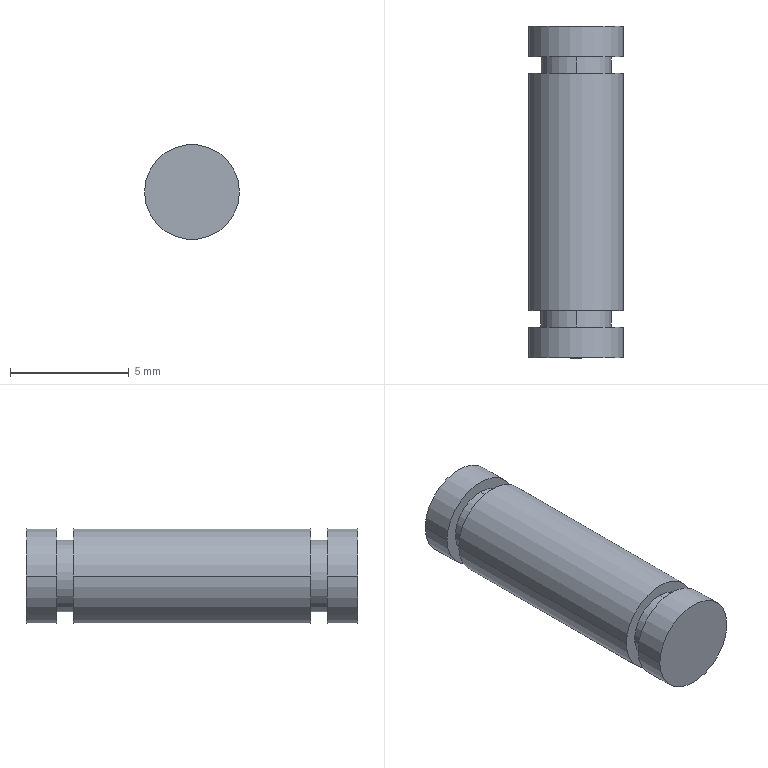Part | NX | 1 solid | 16 faces | box 4 x 14 x 4 mm | volume 168.232 mm3 | cylinder 10 | plane 6 | commonest cylinder face diameters 4 x6 3 x4
STEP:
#1=CARTESIAN_POINT('',(-42.,151.,-84.4));
#2=VERTEX_POINT('',#1);
#3=CARTESIAN_POINT('',(-46.,151.,-84.4));
#4=VERTEX_POINT('',#3);
#5=CARTESIAN_POINT('',(-44.,151.,-84.4));
#6=DIRECTION('',(0.,1.,0.));
#7=DIRECTION('',(-1.,0.,0.));
#8=AXIS2_PLACEMENT_3D('',#5,#6,#7);
#9=CIRCLE('',#8,2.);
#10=EDGE_CURVE('',#2,#4,#9,.T.);
#11=ORIENTED_EDGE('',*,*,#10,.T.);
#12=CARTESIAN_POINT('',(-46.,152.3,-84.4));
#13=VERTEX_POINT('',#12);
#14=CARTESIAN_POINT('',(-46.,165.,-84.4));
#15=DIRECTION('',(0.,1.,0.));
#16=VECTOR('',#15,1000.);
#17=LINE('',#14,#16);
#18=EDGE_CURVE('',#4,#13,#17,.T.);
#19=ORIENTED_EDGE('',*,*,#18,.T.);
#20=CARTESIAN_POINT('',(-42.,152.3,-84.4));
#21=VERTEX_POINT('',#20);
#22=CARTESIAN_POINT('',(-44.,152.3,-84.4));
#23=DIRECTION('',(0.,1.,0.));
#24=DIRECTION('',(-1.,0.,0.));
#25=AXIS2_PLACEMENT_3D('',#22,#23,#24);
#26=CIRCLE('',#25,2.);
#27=EDGE_CURVE('',#21,#13,#26,.T.);
#28=ORIENTED_EDGE('',*,*,#27,.F.);
#29=CARTESIAN_POINT('',(-42.,165.,-84.4));
#30=DIRECTION('',(0.,1.,0.));
#31=VECTOR('',#30,1000.);
#32=LINE('',#29,#31);
#33=EDGE_CURVE('',#2,#21,#32,.T.);
#34=ORIENTED_EDGE('',*,*,#33,.F.);
#35=EDGE_LOOP('',(#11,#19,#28,#34));
#36=FACE_BOUND('',#35,.T.);
#37=CARTESIAN_POINT('',(-44.,165.,-84.4));
#38=DIRECTION('',(0.,1.,0.));
#39=DIRECTION('',(-1.,0.,0.));
#40=AXIS2_PLACEMENT_3D('',#37,#38,#39);
#41=CYLINDRICAL_SURFACE('',#40,2.);
#42=ADVANCED_FACE('',(#36),#41,.T.);
#43=CARTESIAN_POINT('',(-42.,163.7,-84.4));
#44=VERTEX_POINT('',#43);
#45=CARTESIAN_POINT('',(-46.,163.7,-84.4));
#46=VERTEX_POINT('',#45);
#47=CARTESIAN_POINT('',(-44.,163.7,-84.4));
#48=DIRECTION('',(0.,1.,0.));
#49=DIRECTION('',(-1.,0.,0.));
#50=AXIS2_PLACEMENT_3D('',#47,#48,#49);
#51=CIRCLE('',#50,2.);
#52=EDGE_CURVE('',#44,#46,#51,.T.);
#53=ORIENTED_EDGE('',*,*,#52,.T.);
#54=CARTESIAN_POINT('',(-46.,165.,-84.4));
#55=VERTEX_POINT('',#54);
#56=CARTESIAN_POINT('',(-46.,165.,-84.4));
#57=DIRECTION('',(0.,1.,0.));
#58=VECTOR('',#57,1000.);
#59=LINE('',#56,#58);
#60=EDGE_CURVE('',#55,#46,#59,.F.);
#61=ORIENTED_EDGE('',*,*,#60,.F.);
#62=CARTESIAN_POINT('',(-42.,165.,-84.4));
#63=VERTEX_POINT('',#62);
#64=CARTESIAN_POINT('',(-44.,165.,-84.4));
#65=DIRECTION('',(0.,1.,0.));
#66=DIRECTION('',(-1.,0.,0.));
#67=AXIS2_PLACEMENT_3D('',#64,#65,#66);
#68=CIRCLE('',#67,2.);
#69=EDGE_CURVE('',#63,#55,#68,.T.);
#70=ORIENTED_EDGE('',*,*,#69,.F.);
#71=CARTESIAN_POINT('',(-42.,165.,-84.4));
#72=DIRECTION('',(0.,1.,0.));
#73=VECTOR('',#72,1000.);
#74=LINE('',#71,#73);
#75=EDGE_CURVE('',#63,#44,#74,.F.);
#76=ORIENTED_EDGE('',*,*,#75,.T.);
#77=EDGE_LOOP('',(#53,#61,#70,#76));
#78=FACE_BOUND('',#77,.T.);
#79=CARTESIAN_POINT('',(-44.,165.,-84.4));
#80=DIRECTION('',(0.,1.,0.));
#81=DIRECTION('',(-1.,0.,0.));
#82=AXIS2_PLACEMENT_3D('',#79,#80,#81);
#83=CYLINDRICAL_SURFACE('',#82,2.);
#84=ADVANCED_FACE('',(#78),#83,.T.);
#85=CARTESIAN_POINT('',(-42.,153.,-84.4));
#86=VERTEX_POINT('',#85);
#87=CARTESIAN_POINT('',(-46.,153.,-84.4));
#88=VERTEX_POINT('',#87);
#89=CARTESIAN_POINT('',(-44.,153.,-84.4));
#90=DIRECTION('',(0.,1.,0.));
#91=DIRECTION('',(-1.,0.,0.));
#92=AXIS2_PLACEMENT_3D('',#89,#90,#91);
#93=CIRCLE('',#92,2.);
#94=EDGE_CURVE('',#86,#88,#93,.T.);
#95=ORIENTED_EDGE('',*,*,#94,.T.);
#96=CARTESIAN_POINT('',(-46.,163.,-84.4));
#97=VERTEX_POINT('',#96);
#98=CARTESIAN_POINT('',(-46.,165.,-84.4));
#99=DIRECTION('',(0.,1.,0.));
#100=VECTOR('',#99,1000.);
#101=LINE('',#98,#100);
#102=EDGE_CURVE('',#97,#88,#101,.F.);
#103=ORIENTED_EDGE('',*,*,#102,.F.);
#104=CARTESIAN_POINT('',(-42.,163.,-84.4));
#105=VERTEX_POINT('',#104);
#106=CARTESIAN_POINT('',(-44.,163.,-84.4));
#107=DIRECTION('',(0.,1.,0.));
#108=DIRECTION('',(-1.,0.,0.));
#109=AXIS2_PLACEMENT_3D('',#106,#107,#108);
#110=CIRCLE('',#109,2.);
#111=EDGE_CURVE('',#105,#97,#110,.T.);
#112=ORIENTED_EDGE('',*,*,#111,.F.);
#113=CARTESIAN_POINT('',(-42.,165.,-84.4));
#114=DIRECTION('',(0.,1.,0.));
#115=VECTOR('',#114,1000.);
#116=LINE('',#113,#115);
#117=EDGE_CURVE('',#105,#86,#116,.F.);
#118=ORIENTED_EDGE('',*,*,#117,.T.);
#119=EDGE_LOOP('',(#95,#103,#112,#118));
#120=FACE_BOUND('',#119,.T.);
#121=CARTESIAN_POINT('',(-44.,165.,-84.4));
#122=DIRECTION('',(0.,1.,0.));
#123=DIRECTION('',(-1.,0.,0.));
#124=AXIS2_PLACEMENT_3D('',#121,#122,#123);
#125=CYLINDRICAL_SURFACE('',#124,2.);
#126=ADVANCED_FACE('',(#120),#125,.T.);
#127=ORIENTED_EDGE('',*,*,#52,.F.);
#128=CARTESIAN_POINT('',(-44.,163.7,-84.4));
#129=DIRECTION('',(0.,1.,0.));
#130=DIRECTION('',(-1.,0.,0.));
#131=AXIS2_PLACEMENT_3D('',#128,#129,#130);
#132=CIRCLE('',#131,2.);
#133=EDGE_CURVE('',#46,#44,#132,.T.);
#134=ORIENTED_EDGE('',*,*,#133,.F.);
#135=EDGE_LOOP('',(#127,#134));
#136=FACE_BOUND('',#135,.T.);
#137=CARTESIAN_POINT('',(-44.,163.7,-82.9));
#138=VERTEX_POINT('',#137);
#139=CARTESIAN_POINT('',(-44.,163.7,-85.9));
#140=VERTEX_POINT('',#139);
#141=CARTESIAN_POINT('',(-44.,163.7,-84.4));
#142=DIRECTION('',(0.,1.,0.));
#143=DIRECTION('',(1.,0.,0.));
#144=AXIS2_PLACEMENT_3D('',#141,#142,#143);
#145=CIRCLE('',#144,1.5);
#146=EDGE_CURVE('',#138,#140,#145,.T.);
#147=ORIENTED_EDGE('',*,*,#146,.T.);
#148=CARTESIAN_POINT('',(-44.,163.7,-84.4));
#149=DIRECTION('',(0.,1.,0.));
#150=DIRECTION('',(1.,0.,0.));
#151=AXIS2_PLACEMENT_3D('',#148,#149,#150);
#152=CIRCLE('',#151,1.5);
#153=EDGE_CURVE('',#140,#138,#152,.T.);
#154=ORIENTED_EDGE('',*,*,#153,.T.);
#155=EDGE_LOOP('',(#147,#154));
#156=FACE_BOUND('',#155,.T.);
#157=CARTESIAN_POINT('',(-41.314,163.7,-84.4));
#158=DIRECTION('',(0.,1.,0.));
#159=DIRECTION('',(0.,0.,-1.));
#160=AXIS2_PLACEMENT_3D('',#157,#158,#159);
#161=PLANE('',#160);
#162=ADVANCED_FACE('',(#136,#156),#161,.F.);
#163=ORIENTED_EDGE('',*,*,#146,.F.);
#164=CARTESIAN_POINT('',(-44.,163.,-82.9));
#165=VERTEX_POINT('',#164);
#166=CARTESIAN_POINT('',(-44.,163.35,-82.9));
#167=DIRECTION('',(0.,1.,0.));
#168=VECTOR('',#167,1000.);
#169=LINE('',#166,#168);
#170=EDGE_CURVE('',#165,#138,#169,.T.);
#171=ORIENTED_EDGE('',*,*,#170,.F.);
#172=CARTESIAN_POINT('',(-44.,163.,-85.9));
#173=VERTEX_POINT('',#172);
#174=CARTESIAN_POINT('',(-44.,163.,-84.4));
#175=DIRECTION('',(0.,1.,0.));
#176=DIRECTION('',(1.,0.,0.));
#177=AXIS2_PLACEMENT_3D('',#174,#175,#176);
#178=CIRCLE('',#177,1.5);
#179=EDGE_CURVE('',#165,#173,#178,.T.);
#180=ORIENTED_EDGE('',*,*,#179,.T.);
#181=CARTESIAN_POINT('',(-44.,163.35,-85.9));
#182=DIRECTION('',(0.,1.,0.));
#183=VECTOR('',#182,1000.);
#184=LINE('',#181,#183);
#185=EDGE_CURVE('',#173,#140,#184,.T.);
#186=ORIENTED_EDGE('',*,*,#185,.T.);
#187=EDGE_LOOP('',(#163,#171,#180,#186));
#188=FACE_BOUND('',#187,.T.);
#189=CARTESIAN_POINT('',(-44.,163.35,-84.4));
#190=DIRECTION('',(0.,1.,0.));
#191=DIRECTION('',(0.,0.,1.));
#192=AXIS2_PLACEMENT_3D('',#189,#190,#191);
#193=CYLINDRICAL_SURFACE('',#192,1.5);
#194=ADVANCED_FACE('',(#188),#193,.T.);
#195=CARTESIAN_POINT('',(-44.,163.,-84.4));
#196=DIRECTION('',(0.,1.,0.));
#197=DIRECTION('',(-1.,0.,0.));
#198=AXIS2_PLACEMENT_3D('',#195,#196,#197);
#199=CIRCLE('',#198,2.);
#200=EDGE_CURVE('',#97,#105,#199,.T.);
#201=ORIENTED_EDGE('',*,*,#200,.T.);
#202=ORIENTED_EDGE('',*,*,#111,.T.);
#203=EDGE_LOOP('',(#201,#202));
#204=FACE_BOUND('',#203,.T.);
#205=ORIENTED_EDGE('',*,*,#179,.F.);
#206=CARTESIAN_POINT('',(-44.,163.,-84.4));
#207=DIRECTION('',(0.,1.,0.));
#208=DIRECTION('',(1.,0.,0.));
#209=AXIS2_PLACEMENT_3D('',#206,#207,#208);
#210=CIRCLE('',#209,1.5);
#211=EDGE_CURVE('',#173,#165,#210,.T.);
#212=ORIENTED_EDGE('',*,*,#211,.F.);
#213=EDGE_LOOP('',(#205,#212));
#214=FACE_BOUND('',#213,.T.);
#215=CARTESIAN_POINT('',(-42.25,163.,-84.4));
#216=DIRECTION('',(0.,-1.,0.));
#217=DIRECTION('',(-1.,0.,0.));
#218=AXIS2_PLACEMENT_3D('',#215,#216,#217);
#219=PLANE('',#218);
#220=ADVANCED_FACE('',(#204,#214),#219,.F.);
#221=ORIENTED_EDGE('',*,*,#94,.F.);
#222=CARTESIAN_POINT('',(-44.,153.,-84.4));
#223=DIRECTION('',(0.,1.,0.));
#224=DIRECTION('',(-1.,0.,0.));
#225=AXIS2_PLACEMENT_3D('',#222,#223,#224);
#226=CIRCLE('',#225,2.);
#227=EDGE_CURVE('',#88,#86,#226,.T.);
#228=ORIENTED_EDGE('',*,*,#227,.F.);
#229=EDGE_LOOP('',(#221,#228));
#230=FACE_BOUND('',#229,.T.);
#231=CARTESIAN_POINT('',(-44.,153.,-85.9));
#232=VERTEX_POINT('',#231);
#233=CARTESIAN_POINT('',(-44.,153.,-82.9));
#234=VERTEX_POINT('',#233);
#235=CARTESIAN_POINT('',(-44.,153.,-84.4));
#236=DIRECTION('',(0.,1.,0.));
#237=DIRECTION('',(0.,0.,1.));
#238=AXIS2_PLACEMENT_3D('',#235,#236,#237);
#239=CIRCLE('',#238,1.5);
#240=EDGE_CURVE('',#232,#234,#239,.T.);
#241=ORIENTED_EDGE('',*,*,#240,.T.);
#242=CARTESIAN_POINT('',(-44.,153.,-84.4));
#243=DIRECTION('',(0.,1.,0.));
#244=DIRECTION('',(0.,0.,1.));
#245=AXIS2_PLACEMENT_3D('',#242,#243,#244);
#246=CIRCLE('',#245,1.5);
#247=EDGE_CURVE('',#234,#232,#246,.T.);
#248=ORIENTED_EDGE('',*,*,#247,.T.);
#249=EDGE_LOOP('',(#241,#248));
#250=FACE_BOUND('',#249,.T.);
#251=CARTESIAN_POINT('',(-42.25,153.,-84.4));
#252=DIRECTION('',(0.,1.,0.));
#253=DIRECTION('',(0.,0.,-1.));
#254=AXIS2_PLACEMENT_3D('',#251,#252,#253);
#255=PLANE('',#254);
#256=ADVANCED_FACE('',(#230,#250),#255,.F.);
#257=ORIENTED_EDGE('',*,*,#240,.F.);
#258=CARTESIAN_POINT('',(-44.,152.3,-85.9));
#259=VERTEX_POINT('',#258);
#260=CARTESIAN_POINT('',(-44.,154.65,-85.9));
#261=DIRECTION('',(0.,1.,0.));
#262=VECTOR('',#261,1000.);
#263=LINE('',#260,#262);
#264=EDGE_CURVE('',#259,#232,#263,.T.);
#265=ORIENTED_EDGE('',*,*,#264,.F.);
#266=CARTESIAN_POINT('',(-44.,152.3,-82.9));
#267=VERTEX_POINT('',#266);
#268=CARTESIAN_POINT('',(-44.,152.3,-84.4));
#269=DIRECTION('',(0.,1.,0.));
#270=DIRECTION('',(0.,0.,1.));
#271=AXIS2_PLACEMENT_3D('',#268,#269,#270);
#272=CIRCLE('',#271,1.5);
#273=EDGE_CURVE('',#259,#267,#272,.T.);
#274=ORIENTED_EDGE('',*,*,#273,.T.);
#275=CARTESIAN_POINT('',(-44.,154.65,-82.9));
#276=DIRECTION('',(0.,1.,0.));
#277=VECTOR('',#276,1000.);
#278=LINE('',#275,#277);
#279=EDGE_CURVE('',#267,#234,#278,.T.);
#280=ORIENTED_EDGE('',*,*,#279,.T.);
#281=EDGE_LOOP('',(#257,#265,#274,#280));
#282=FACE_BOUND('',#281,.T.);
#283=CARTESIAN_POINT('',(-44.,154.65,-84.4));
#284=DIRECTION('',(0.,1.,0.));
#285=DIRECTION('',(0.,0.,1.));
#286=AXIS2_PLACEMENT_3D('',#283,#284,#285);
#287=CYLINDRICAL_SURFACE('',#286,1.5);
#288=ADVANCED_FACE('',(#282),#287,.T.);
#289=ORIENTED_EDGE('',*,*,#27,.T.);
#290=CARTESIAN_POINT('',(-44.,152.3,-84.4));
#291=DIRECTION('',(0.,1.,0.));
#292=DIRECTION('',(-1.,0.,0.));
#293=AXIS2_PLACEMENT_3D('',#290,#291,#292);
#294=CIRCLE('',#293,2.);
#295=EDGE_CURVE('',#13,#21,#294,.T.);
#296=ORIENTED_EDGE('',*,*,#295,.T.);
#297=EDGE_LOOP('',(#289,#296));
#298=FACE_BOUND('',#297,.T.);
#299=ORIENTED_EDGE('',*,*,#273,.F.);
#300=CARTESIAN_POINT('',(-44.,152.3,-84.4));
#301=DIRECTION('',(0.,1.,0.));
#302=DIRECTION('',(0.,0.,1.));
#303=AXIS2_PLACEMENT_3D('',#300,#301,#302);
#304=CIRCLE('',#303,1.5);
#305=EDGE_CURVE('',#267,#259,#304,.T.);
#306=ORIENTED_EDGE('',*,*,#305,.F.);
#307=EDGE_LOOP('',(#299,#306));
#308=FACE_BOUND('',#307,.T.);
#309=CARTESIAN_POINT('',(-41.396,152.3,-84.4));
#310=DIRECTION('',(0.,1.,0.));
#311=DIRECTION('',(0.,0.,-1.));
#312=AXIS2_PLACEMENT_3D('',#309,#310,#311);
#313=PLANE('',#312);
#314=ADVANCED_FACE('',(#298,#308),#313,.T.);
#315=ORIENTED_EDGE('',*,*,#200,.F.);
#316=ORIENTED_EDGE('',*,*,#102,.T.);
#317=ORIENTED_EDGE('',*,*,#227,.T.);
#318=ORIENTED_EDGE('',*,*,#117,.F.);
#319=EDGE_LOOP('',(#315,#316,#317,#318));
#320=FACE_BOUND('',#319,.T.);
#321=CARTESIAN_POINT('',(-44.,165.,-84.4));
#322=DIRECTION('',(0.,1.,0.));
#323=DIRECTION('',(-1.,0.,0.));
#324=AXIS2_PLACEMENT_3D('',#321,#322,#323);
#325=CYLINDRICAL_SURFACE('',#324,2.);
#326=ADVANCED_FACE('',(#320),#325,.T.);
#327=ORIENTED_EDGE('',*,*,#279,.F.);
#328=ORIENTED_EDGE('',*,*,#305,.T.);
#329=ORIENTED_EDGE('',*,*,#264,.T.);
#330=ORIENTED_EDGE('',*,*,#247,.F.);
#331=EDGE_LOOP('',(#327,#328,#329,#330));
#332=FACE_BOUND('',#331,.T.);
#333=CARTESIAN_POINT('',(-44.,154.65,-84.4));
#334=DIRECTION('',(0.,1.,0.));
#335=DIRECTION('',(0.,0.,1.));
#336=AXIS2_PLACEMENT_3D('',#333,#334,#335);
#337=CYLINDRICAL_SURFACE('',#336,1.5);
#338=ADVANCED_FACE('',(#332),#337,.T.);
#339=ORIENTED_EDGE('',*,*,#60,.T.);
#340=ORIENTED_EDGE('',*,*,#133,.T.);
#341=ORIENTED_EDGE('',*,*,#75,.F.);
#342=CARTESIAN_POINT('',(-44.,165.,-84.4));
#343=DIRECTION('',(0.,1.,0.));
#344=DIRECTION('',(-1.,0.,0.));
#345=AXIS2_PLACEMENT_3D('',#342,#343,#344);
#346=CIRCLE('',#345,2.);
#347=EDGE_CURVE('',#55,#63,#346,.T.);
#348=ORIENTED_EDGE('',*,*,#347,.F.);
#349=EDGE_LOOP('',(#339,#340,#341,#348));
#350=FACE_BOUND('',#349,.T.);
#351=CARTESIAN_POINT('',(-44.,165.,-84.4));
#352=DIRECTION('',(0.,1.,0.));
#353=DIRECTION('',(-1.,0.,0.));
#354=AXIS2_PLACEMENT_3D('',#351,#352,#353);
#355=CYLINDRICAL_SURFACE('',#354,2.);
#356=ADVANCED_FACE('',(#350),#355,.T.);
#357=ORIENTED_EDGE('',*,*,#170,.T.);
#358=ORIENTED_EDGE('',*,*,#153,.F.);
#359=ORIENTED_EDGE('',*,*,#185,.F.);
#360=ORIENTED_EDGE('',*,*,#211,.T.);
#361=EDGE_LOOP('',(#357,#358,#359,#360));
#362=FACE_BOUND('',#361,.T.);
#363=CARTESIAN_POINT('',(-44.,163.35,-84.4));
#364=DIRECTION('',(0.,1.,0.));
#365=DIRECTION('',(0.,0.,1.));
#366=AXIS2_PLACEMENT_3D('',#363,#364,#365);
#367=CYLINDRICAL_SURFACE('',#366,1.5);
#368=ADVANCED_FACE('',(#362),#367,.T.);
#369=ORIENTED_EDGE('',*,*,#33,.T.);
#370=ORIENTED_EDGE('',*,*,#295,.F.);
#371=ORIENTED_EDGE('',*,*,#18,.F.);
#372=CARTESIAN_POINT('',(-44.,151.,-84.4));
#373=DIRECTION('',(0.,1.,0.));
#374=DIRECTION('',(-1.,0.,0.));
#375=AXIS2_PLACEMENT_3D('',#372,#373,#374);
#376=CIRCLE('',#375,2.);
#377=EDGE_CURVE('',#4,#2,#376,.T.);
#378=ORIENTED_EDGE('',*,*,#377,.T.);
#379=EDGE_LOOP('',(#369,#370,#371,#378));
#380=FACE_BOUND('',#379,.T.);
#381=CARTESIAN_POINT('',(-44.,165.,-84.4));
#382=DIRECTION('',(0.,1.,0.));
#383=DIRECTION('',(-1.,0.,0.));
#384=AXIS2_PLACEMENT_3D('',#381,#382,#383);
#385=CYLINDRICAL_SURFACE('',#384,2.);
#386=ADVANCED_FACE('',(#380),#385,.T.);
#387=ORIENTED_EDGE('',*,*,#10,.F.);
#388=ORIENTED_EDGE('',*,*,#377,.F.);
#389=EDGE_LOOP('',(#387,#388));
#390=FACE_BOUND('',#389,.T.);
#391=CARTESIAN_POINT('',(-42.256,151.,-78.065));
#392=DIRECTION('',(0.,1.,0.));
#393=DIRECTION('',(0.,0.,-1.));
#394=AXIS2_PLACEMENT_3D('',#391,#392,#393);
#395=PLANE('',#394);
#396=ADVANCED_FACE('',(#390),#395,.F.);
#397=ORIENTED_EDGE('',*,*,#69,.T.);
#398=ORIENTED_EDGE('',*,*,#347,.T.);
#399=EDGE_LOOP('',(#397,#398));
#400=FACE_BOUND('',#399,.T.);
#401=CARTESIAN_POINT('',(-42.256,165.,-78.065));
#402=DIRECTION('',(0.,1.,0.));
#403=DIRECTION('',(0.,0.,-1.));
#404=AXIS2_PLACEMENT_3D('',#401,#402,#403);
#405=PLANE('',#404);
#406=ADVANCED_FACE('',(#400),#405,.T.);
#407=CLOSED_SHELL('',(#42,#84,#126,#162,#194,#220,#256,#288,#314,#326,#338,#356,#368,#386,#396,#406));
#408=MANIFOLD_SOLID_BREP('',#407);
#409=(LENGTH_UNIT()NAMED_UNIT(*)SI_UNIT(.MILLI.,.METRE.));
#410=UNCERTAINTY_MEASURE_WITH_UNIT(LENGTH_MEASURE(0.00001),#409,'','');
#411=(NAMED_UNIT(*)PLANE_ANGLE_UNIT()SI_UNIT($,.RADIAN.));
#412=(NAMED_UNIT(*)SI_UNIT($,.STERADIAN.)SOLID_ANGLE_UNIT());
#413=(GEOMETRIC_REPRESENTATION_CONTEXT(3)GLOBAL_UNCERTAINTY_ASSIGNED_CONTEXT((#410))GLOBAL_UNIT_ASSIGNED_CONTEXT((#409,#411,#412))REPRESENTATION_CONTEXT('',''));
#414=ADVANCED_BREP_SHAPE_REPRESENTATION('',(#408),#413);